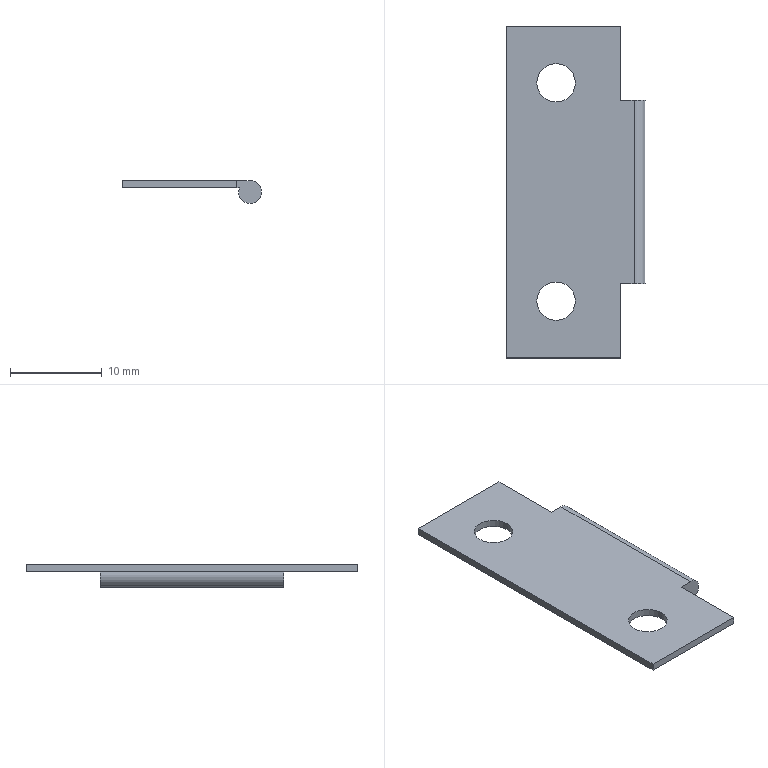Part | STEP file | 1.5 inch micro hinge plate-right | 1 solid | 15 faces | box 15.15 x 36.2 x 2.5 mm | volume 446.218 mm3 | plane 9 | cylinder 6 | commonest cylinder face diameters 4.2 x4 2.5 x2
STEP:
#1=CARTESIAN_POINT('',(0.,0.,0.));
#2=DIRECTION('',(0.,0.,1.));
#3=DIRECTION('',(1.,0.,0.));
#4=AXIS2_PLACEMENT_3D('',#1,#2,#3);
#5=CARTESIAN_POINT('',(-3.65,11.9,0.4));
#6=VERTEX_POINT('',#5);
#7=CARTESIAN_POINT('',(-3.65,11.9,-0.4));
#8=VERTEX_POINT('',#7);
#9=CARTESIAN_POINT('',(-3.65,11.9,-0.4));
#10=DIRECTION('',(0.,0.,-1.));
#11=VECTOR('',#10,1.);
#12=LINE('',#9,#11);
#13=CARTESIAN_POINT('',(-1.55,11.9,-0.4));
#14=DIRECTION('',(0.,0.,-1.));
#15=DIRECTION('',(-1.,0.,0.));
#16=AXIS2_PLACEMENT_3D('',#13,#14,#15);
#17=CYLINDRICAL_SURFACE('',#16,2.1);
#18=CARTESIAN_POINT('',(6.283,0.));
#19=DIRECTION('',(0.,1.));
#20=VECTOR('',#19,1.);
#21=LINE('',#18,#20);
#22=(GEOMETRIC_REPRESENTATION_CONTEXT(2)PARAMETRIC_REPRESENTATION_CONTEXT()REPRESENTATION_CONTEXT('',''));
#23=DEFINITIONAL_REPRESENTATION('',(#21),#22);
#24=PCURVE('',#17,#23);
#25=CARTESIAN_POINT('',(-1.55,11.9,-0.4));
#26=DIRECTION('',(0.,0.,-1.));
#27=DIRECTION('',(-1.,0.,0.));
#28=AXIS2_PLACEMENT_3D('',#25,#26,#27);
#29=CYLINDRICAL_SURFACE('',#28,2.1);
#30=CARTESIAN_POINT('',(0.,0.));
#31=DIRECTION('',(0.,1.));
#32=VECTOR('',#31,1.);
#33=LINE('',#30,#32);
#34=(GEOMETRIC_REPRESENTATION_CONTEXT(2)PARAMETRIC_REPRESENTATION_CONTEXT()REPRESENTATION_CONTEXT('',''));
#35=DEFINITIONAL_REPRESENTATION('',(#33),#34);
#36=PCURVE('',#29,#35);
#37=SURFACE_CURVE('',#12,(#24,#36),.PCURVE_S1.);
#38=EDGE_CURVE('',#6,#8,#37,.T.);
#39=ORIENTED_EDGE('',*,*,#38,.T.);
#40=CARTESIAN_POINT('',(0.55,11.9,-0.4));
#41=VERTEX_POINT('',#40);
#42=CARTESIAN_POINT('',(-1.55,11.9,-0.4));
#43=DIRECTION('',(0.,0.,-1.));
#44=DIRECTION('',(-1.,0.,0.));
#45=AXIS2_PLACEMENT_3D('',#42,#43,#44);
#46=CIRCLE('',#45,2.1);
#47=CARTESIAN_POINT('',(0.,0.));
#48=DIRECTION('',(1.,0.));
#49=VECTOR('',#48,1.);
#50=LINE('',#47,#49);
#51=(GEOMETRIC_REPRESENTATION_CONTEXT(2)PARAMETRIC_REPRESENTATION_CONTEXT()REPRESENTATION_CONTEXT('',''));
#52=DEFINITIONAL_REPRESENTATION('',(#50),#51);
#53=PCURVE('',#17,#52);
#54=CARTESIAN_POINT('',(0.,0.,-0.4));
#55=DIRECTION('',(0.,0.,-1.));
#56=DIRECTION('',(-1.,0.,0.));
#57=AXIS2_PLACEMENT_3D('',#54,#55,#56);
#58=PLANE('',#57);
#59=CARTESIAN_POINT('',(1.55,11.9));
#60=DIRECTION('',(1.,0.));
#61=AXIS2_PLACEMENT_2D('',#59,#60);
#62=CIRCLE('',#61,2.1);
#63=(GEOMETRIC_REPRESENTATION_CONTEXT(2)PARAMETRIC_REPRESENTATION_CONTEXT()REPRESENTATION_CONTEXT('',''));
#64=DEFINITIONAL_REPRESENTATION('',(#62),#63);
#65=PCURVE('',#58,#64);
#66=SURFACE_CURVE('',#46,(#53,#65),.PCURVE_S1.);
#67=EDGE_CURVE('',#41,#8,#66,.T.);
#68=ORIENTED_EDGE('',*,*,#67,.F.);
#69=CARTESIAN_POINT('',(0.55,11.9,0.4));
#70=VERTEX_POINT('',#69);
#71=CARTESIAN_POINT('',(0.55,11.9,-0.4));
#72=DIRECTION('',(0.,0.,-1.));
#73=VECTOR('',#72,1.);
#74=LINE('',#71,#73);
#75=CARTESIAN_POINT('',(3.142,0.));
#76=DIRECTION('',(0.,1.));
#77=VECTOR('',#76,1.);
#78=LINE('',#75,#77);
#79=(GEOMETRIC_REPRESENTATION_CONTEXT(2)PARAMETRIC_REPRESENTATION_CONTEXT()REPRESENTATION_CONTEXT('',''));
#80=DEFINITIONAL_REPRESENTATION('',(#78),#79);
#81=PCURVE('',#17,#80);
#82=CARTESIAN_POINT('',(3.142,0.));
#83=DIRECTION('',(0.,1.));
#84=VECTOR('',#83,1.);
#85=LINE('',#82,#84);
#86=(GEOMETRIC_REPRESENTATION_CONTEXT(2)PARAMETRIC_REPRESENTATION_CONTEXT()REPRESENTATION_CONTEXT('',''));
#87=DEFINITIONAL_REPRESENTATION('',(#85),#86);
#88=PCURVE('',#29,#87);
#89=SURFACE_CURVE('',#74,(#81,#88),.PCURVE_S1.);
#90=EDGE_CURVE('',#70,#41,#89,.T.);
#91=ORIENTED_EDGE('',*,*,#90,.F.);
#92=CARTESIAN_POINT('',(-1.55,11.9,0.4));
#93=DIRECTION('',(0.,0.,-1.));
#94=DIRECTION('',(-1.,0.,0.));
#95=AXIS2_PLACEMENT_3D('',#92,#93,#94);
#96=CIRCLE('',#95,2.1);
#97=CARTESIAN_POINT('',(0.,-0.8));
#98=DIRECTION('',(1.,0.));
#99=VECTOR('',#98,1.);
#100=LINE('',#97,#99);
#101=(GEOMETRIC_REPRESENTATION_CONTEXT(2)PARAMETRIC_REPRESENTATION_CONTEXT()REPRESENTATION_CONTEXT('',''));
#102=DEFINITIONAL_REPRESENTATION('',(#100),#101);
#103=PCURVE('',#17,#102);
#104=CARTESIAN_POINT('',(0.,0.,0.4));
#105=DIRECTION('',(0.,0.,-1.));
#106=DIRECTION('',(-1.,0.,0.));
#107=AXIS2_PLACEMENT_3D('',#104,#105,#106);
#108=PLANE('',#107);
#109=CARTESIAN_POINT('',(1.55,11.9));
#110=DIRECTION('',(1.,0.));
#111=AXIS2_PLACEMENT_2D('',#109,#110);
#112=CIRCLE('',#111,2.1);
#113=(GEOMETRIC_REPRESENTATION_CONTEXT(2)PARAMETRIC_REPRESENTATION_CONTEXT()REPRESENTATION_CONTEXT('',''));
#114=DEFINITIONAL_REPRESENTATION('',(#112),#113);
#115=PCURVE('',#108,#114);
#116=SURFACE_CURVE('',#96,(#103,#115),.PCURVE_S1.);
#117=EDGE_CURVE('',#70,#6,#116,.T.);
#118=ORIENTED_EDGE('',*,*,#117,.T.);
#119=EDGE_LOOP('',(#39,#68,#91,#118));
#120=FACE_BOUND('',#119,.F.);
#121=ADVANCED_FACE('',(#120),#17,.F.);
#122=CARTESIAN_POINT('',(-3.65,-11.9,0.4));
#123=VERTEX_POINT('',#122);
#124=CARTESIAN_POINT('',(-3.65,-11.9,-0.4));
#125=VERTEX_POINT('',#124);
#126=CARTESIAN_POINT('',(-3.65,-11.9,-0.4));
#127=DIRECTION('',(0.,0.,-1.));
#128=VECTOR('',#127,1.);
#129=LINE('',#126,#128);
#130=CARTESIAN_POINT('',(-1.55,-11.9,-0.4));
#131=DIRECTION('',(0.,0.,-1.));
#132=DIRECTION('',(-1.,0.,0.));
#133=AXIS2_PLACEMENT_3D('',#130,#131,#132);
#134=CYLINDRICAL_SURFACE('',#133,2.1);
#135=CARTESIAN_POINT('',(6.283,0.));
#136=DIRECTION('',(0.,1.));
#137=VECTOR('',#136,1.);
#138=LINE('',#135,#137);
#139=(GEOMETRIC_REPRESENTATION_CONTEXT(2)PARAMETRIC_REPRESENTATION_CONTEXT()REPRESENTATION_CONTEXT('',''));
#140=DEFINITIONAL_REPRESENTATION('',(#138),#139);
#141=PCURVE('',#134,#140);
#142=CARTESIAN_POINT('',(-1.55,-11.9,-0.4));
#143=DIRECTION('',(0.,0.,-1.));
#144=DIRECTION('',(-1.,0.,0.));
#145=AXIS2_PLACEMENT_3D('',#142,#143,#144);
#146=CYLINDRICAL_SURFACE('',#145,2.1);
#147=CARTESIAN_POINT('',(0.,0.));
#148=DIRECTION('',(0.,1.));
#149=VECTOR('',#148,1.);
#150=LINE('',#147,#149);
#151=(GEOMETRIC_REPRESENTATION_CONTEXT(2)PARAMETRIC_REPRESENTATION_CONTEXT()REPRESENTATION_CONTEXT('',''));
#152=DEFINITIONAL_REPRESENTATION('',(#150),#151);
#153=PCURVE('',#146,#152);
#154=SURFACE_CURVE('',#129,(#141,#153),.PCURVE_S1.);
#155=EDGE_CURVE('',#123,#125,#154,.T.);
#156=ORIENTED_EDGE('',*,*,#155,.T.);
#157=CARTESIAN_POINT('',(0.55,-11.9,-0.4));
#158=VERTEX_POINT('',#157);
#159=CARTESIAN_POINT('',(-1.55,-11.9,-0.4));
#160=DIRECTION('',(0.,0.,-1.));
#161=DIRECTION('',(-1.,0.,0.));
#162=AXIS2_PLACEMENT_3D('',#159,#160,#161);
#163=CIRCLE('',#162,2.1);
#164=CARTESIAN_POINT('',(0.,0.));
#165=DIRECTION('',(1.,0.));
#166=VECTOR('',#165,1.);
#167=LINE('',#164,#166);
#168=(GEOMETRIC_REPRESENTATION_CONTEXT(2)PARAMETRIC_REPRESENTATION_CONTEXT()REPRESENTATION_CONTEXT('',''));
#169=DEFINITIONAL_REPRESENTATION('',(#167),#168);
#170=PCURVE('',#134,#169);
#171=CARTESIAN_POINT('',(1.55,-11.9));
#172=DIRECTION('',(1.,0.));
#173=AXIS2_PLACEMENT_2D('',#171,#172);
#174=CIRCLE('',#173,2.1);
#175=(GEOMETRIC_REPRESENTATION_CONTEXT(2)PARAMETRIC_REPRESENTATION_CONTEXT()REPRESENTATION_CONTEXT('',''));
#176=DEFINITIONAL_REPRESENTATION('',(#174),#175);
#177=PCURVE('',#58,#176);
#178=SURFACE_CURVE('',#163,(#170,#177),.PCURVE_S1.);
#179=EDGE_CURVE('',#158,#125,#178,.T.);
#180=ORIENTED_EDGE('',*,*,#179,.F.);
#181=CARTESIAN_POINT('',(0.55,-11.9,0.4));
#182=VERTEX_POINT('',#181);
#183=CARTESIAN_POINT('',(0.55,-11.9,-0.4));
#184=DIRECTION('',(0.,0.,-1.));
#185=VECTOR('',#184,1.);
#186=LINE('',#183,#185);
#187=CARTESIAN_POINT('',(3.142,0.));
#188=DIRECTION('',(0.,1.));
#189=VECTOR('',#188,1.);
#190=LINE('',#187,#189);
#191=(GEOMETRIC_REPRESENTATION_CONTEXT(2)PARAMETRIC_REPRESENTATION_CONTEXT()REPRESENTATION_CONTEXT('',''));
#192=DEFINITIONAL_REPRESENTATION('',(#190),#191);
#193=PCURVE('',#134,#192);
#194=CARTESIAN_POINT('',(3.142,0.));
#195=DIRECTION('',(0.,1.));
#196=VECTOR('',#195,1.);
#197=LINE('',#194,#196);
#198=(GEOMETRIC_REPRESENTATION_CONTEXT(2)PARAMETRIC_REPRESENTATION_CONTEXT()REPRESENTATION_CONTEXT('',''));
#199=DEFINITIONAL_REPRESENTATION('',(#197),#198);
#200=PCURVE('',#146,#199);
#201=SURFACE_CURVE('',#186,(#193,#200),.PCURVE_S1.);
#202=EDGE_CURVE('',#182,#158,#201,.T.);
#203=ORIENTED_EDGE('',*,*,#202,.F.);
#204=CARTESIAN_POINT('',(-1.55,-11.9,0.4));
#205=DIRECTION('',(0.,0.,-1.));
#206=DIRECTION('',(-1.,0.,0.));
#207=AXIS2_PLACEMENT_3D('',#204,#205,#206);
#208=CIRCLE('',#207,2.1);
#209=CARTESIAN_POINT('',(0.,-0.8));
#210=DIRECTION('',(1.,0.));
#211=VECTOR('',#210,1.);
#212=LINE('',#209,#211);
#213=(GEOMETRIC_REPRESENTATION_CONTEXT(2)PARAMETRIC_REPRESENTATION_CONTEXT()REPRESENTATION_CONTEXT('',''));
#214=DEFINITIONAL_REPRESENTATION('',(#212),#213);
#215=PCURVE('',#134,#214);
#216=CARTESIAN_POINT('',(1.55,-11.9));
#217=DIRECTION('',(1.,0.));
#218=AXIS2_PLACEMENT_2D('',#216,#217);
#219=CIRCLE('',#218,2.1);
#220=(GEOMETRIC_REPRESENTATION_CONTEXT(2)PARAMETRIC_REPRESENTATION_CONTEXT()REPRESENTATION_CONTEXT('',''));
#221=DEFINITIONAL_REPRESENTATION('',(#219),#220);
#222=PCURVE('',#108,#221);
#223=SURFACE_CURVE('',#208,(#215,#222),.PCURVE_S1.);
#224=EDGE_CURVE('',#182,#123,#223,.T.);
#225=ORIENTED_EDGE('',*,*,#224,.T.);
#226=EDGE_LOOP('',(#156,#180,#203,#225));
#227=FACE_BOUND('',#226,.F.);
#228=ADVANCED_FACE('',(#227),#134,.F.);
#229=CARTESIAN_POINT('',(6.95,10.,-2.1));
#230=VERTEX_POINT('',#229);
#231=CARTESIAN_POINT('',(5.784,10.,-0.4));
#232=VERTEX_POINT('',#231);
#233=CARTESIAN_POINT('',(6.95,10.,-0.85));
#234=DIRECTION('',(0.,1.,0.));
#235=DIRECTION('',(0.,0.,1.));
#236=AXIS2_PLACEMENT_3D('',#233,#234,#235);
#237=CIRCLE('',#236,1.25);
#238=CARTESIAN_POINT('',(6.95,18.1,-0.85));
#239=DIRECTION('',(0.,-1.,0.));
#240=DIRECTION('',(0.,0.,-1.));
#241=AXIS2_PLACEMENT_3D('',#238,#239,#240);
#242=CYLINDRICAL_SURFACE('',#241,1.25);
#243=CARTESIAN_POINT('',(9.425,8.1));
#244=DIRECTION('',(-1.,0.));
#245=VECTOR('',#244,1.);
#246=LINE('',#243,#245);
#247=(GEOMETRIC_REPRESENTATION_CONTEXT(2)PARAMETRIC_REPRESENTATION_CONTEXT()REPRESENTATION_CONTEXT('',''));
#248=DEFINITIONAL_REPRESENTATION('',(#246),#247);
#249=PCURVE('',#242,#248);
#250=CARTESIAN_POINT('',(5.5,10.,0.4));
#251=DIRECTION('',(0.,1.,0.));
#252=DIRECTION('',(0.,0.,1.));
#253=AXIS2_PLACEMENT_3D('',#250,#251,#252);
#254=PLANE('',#253);
#255=CARTESIAN_POINT('',(-1.25,1.45));
#256=DIRECTION('',(1.,0.));
#257=AXIS2_PLACEMENT_2D('',#255,#256);
#258=CIRCLE('',#257,1.25);
#259=(GEOMETRIC_REPRESENTATION_CONTEXT(2)PARAMETRIC_REPRESENTATION_CONTEXT()REPRESENTATION_CONTEXT('',''));
#260=DEFINITIONAL_REPRESENTATION('',(#258),#259);
#261=PCURVE('',#254,#260);
#262=SURFACE_CURVE('',#237,(#249,#261),.PCURVE_S1.);
#263=EDGE_CURVE('',#230,#232,#262,.T.);
#264=ORIENTED_EDGE('',*,*,#263,.F.);
#265=CARTESIAN_POINT('',(6.95,-10.,-2.1));
#266=VERTEX_POINT('',#265);
#267=CARTESIAN_POINT('',(6.95,18.1,-2.1));
#268=DIRECTION('',(0.,-1.,0.));
#269=VECTOR('',#268,1.);
#270=LINE('',#267,#269);
#271=CARTESIAN_POINT('',(6.283,0.));
#272=DIRECTION('',(0.,1.));
#273=VECTOR('',#272,1.);
#274=LINE('',#271,#273);
#275=(GEOMETRIC_REPRESENTATION_CONTEXT(2)PARAMETRIC_REPRESENTATION_CONTEXT()REPRESENTATION_CONTEXT('',''));
#276=DEFINITIONAL_REPRESENTATION('',(#274),#275);
#277=PCURVE('',#242,#276);
#278=CARTESIAN_POINT('',(6.95,18.1,-0.85));
#279=DIRECTION('',(0.,-1.,0.));
#280=DIRECTION('',(0.,0.,-1.));
#281=AXIS2_PLACEMENT_3D('',#278,#279,#280);
#282=CYLINDRICAL_SURFACE('',#281,1.25);
#283=CARTESIAN_POINT('',(0.,0.));
#284=DIRECTION('',(0.,1.));
#285=VECTOR('',#284,1.);
#286=LINE('',#283,#285);
#287=(GEOMETRIC_REPRESENTATION_CONTEXT(2)PARAMETRIC_REPRESENTATION_CONTEXT()REPRESENTATION_CONTEXT('',''));
#288=DEFINITIONAL_REPRESENTATION('',(#286),#287);
#289=PCURVE('',#282,#288);
#290=SURFACE_CURVE('',#270,(#277,#289),.PCURVE_S1.);
#291=EDGE_CURVE('',#230,#266,#290,.T.);
#292=ORIENTED_EDGE('',*,*,#291,.T.);
#293=CARTESIAN_POINT('',(5.784,-10.,-0.4));
#294=VERTEX_POINT('',#293);
#295=CARTESIAN_POINT('',(6.95,-10.,-0.85));
#296=DIRECTION('',(0.,-1.,0.));
#297=DIRECTION('',(0.,0.,-1.));
#298=AXIS2_PLACEMENT_3D('',#295,#296,#297);
#299=CIRCLE('',#298,1.25);
#300=CARTESIAN_POINT('',(0.,28.1));
#301=DIRECTION('',(1.,0.));
#302=VECTOR('',#301,1.);
#303=LINE('',#300,#302);
#304=(GEOMETRIC_REPRESENTATION_CONTEXT(2)PARAMETRIC_REPRESENTATION_CONTEXT()REPRESENTATION_CONTEXT('',''));
#305=DEFINITIONAL_REPRESENTATION('',(#303),#304);
#306=PCURVE('',#242,#305);
#307=CARTESIAN_POINT('',(5.5,-10.,0.4));
#308=DIRECTION('',(0.,-1.,0.));
#309=DIRECTION('',(0.,0.,-1.));
#310=AXIS2_PLACEMENT_3D('',#307,#308,#309);
#311=PLANE('',#310);
#312=CARTESIAN_POINT('',(1.25,1.45));
#313=DIRECTION('',(1.,0.));
#314=AXIS2_PLACEMENT_2D('',#312,#313);
#315=CIRCLE('',#314,1.25);
#316=(GEOMETRIC_REPRESENTATION_CONTEXT(2)PARAMETRIC_REPRESENTATION_CONTEXT()REPRESENTATION_CONTEXT('',''));
#317=DEFINITIONAL_REPRESENTATION('',(#315),#316);
#318=PCURVE('',#311,#317);
#319=SURFACE_CURVE('',#299,(#306,#318),.PCURVE_S1.);
#320=EDGE_CURVE('',#294,#266,#319,.T.);
#321=ORIENTED_EDGE('',*,*,#320,.F.);
#322=CARTESIAN_POINT('',(5.784,18.1,-0.4));
#323=DIRECTION('',(0.,-1.,0.));
#324=VECTOR('',#323,1.);
#325=LINE('',#322,#324);
#326=CARTESIAN_POINT('',(4.344,0.));
#327=DIRECTION('',(0.,1.));
#328=VECTOR('',#327,1.);
#329=LINE('',#326,#328);
#330=(GEOMETRIC_REPRESENTATION_CONTEXT(2)PARAMETRIC_REPRESENTATION_CONTEXT()REPRESENTATION_CONTEXT('',''));
#331=DEFINITIONAL_REPRESENTATION('',(#329),#330);
#332=PCURVE('',#242,#331);
#333=CARTESIAN_POINT('',(-5.784,18.1));
#334=DIRECTION('',(0.,-1.));
#335=VECTOR('',#334,1.);
#336=LINE('',#333,#335);
#337=(GEOMETRIC_REPRESENTATION_CONTEXT(2)PARAMETRIC_REPRESENTATION_CONTEXT()REPRESENTATION_CONTEXT('',''));
#338=DEFINITIONAL_REPRESENTATION('',(#336),#337);
#339=PCURVE('',#58,#338);
#340=SURFACE_CURVE('',#325,(#332,#339),.PCURVE_S1.);
#341=EDGE_CURVE('',#232,#294,#340,.T.);
#342=ORIENTED_EDGE('',*,*,#341,.F.);
#343=EDGE_LOOP('',(#264,#292,#321,#342));
#344=FACE_BOUND('',#343,.T.);
#345=ADVANCED_FACE('',(#344),#242,.T.);
#346=CARTESIAN_POINT('',(-1.55,11.9,-0.4));
#347=DIRECTION('',(0.,0.,-1.));
#348=DIRECTION('',(-1.,0.,0.));
#349=AXIS2_PLACEMENT_3D('',#346,#347,#348);
#350=CIRCLE('',#349,2.1);
#351=CARTESIAN_POINT('',(1.55,11.9));
#352=DIRECTION('',(1.,0.));
#353=AXIS2_PLACEMENT_2D('',#351,#352);
#354=CIRCLE('',#353,2.1);
#355=(GEOMETRIC_REPRESENTATION_CONTEXT(2)PARAMETRIC_REPRESENTATION_CONTEXT()REPRESENTATION_CONTEXT('',''));
#356=DEFINITIONAL_REPRESENTATION('',(#354),#355);
#357=PCURVE('',#58,#356);
#358=CARTESIAN_POINT('',(0.,0.));
#359=DIRECTION('',(1.,0.));
#360=VECTOR('',#359,1.);
#361=LINE('',#358,#360);
#362=(GEOMETRIC_REPRESENTATION_CONTEXT(2)PARAMETRIC_REPRESENTATION_CONTEXT()REPRESENTATION_CONTEXT('',''));
#363=DEFINITIONAL_REPRESENTATION('',(#361),#362);
#364=PCURVE('',#29,#363);
#365=SURFACE_CURVE('',#350,(#357,#364),.PCURVE_S1.);
#366=EDGE_CURVE('',#8,#41,#365,.T.);
#367=ORIENTED_EDGE('',*,*,#366,.F.);
#368=ORIENTED_EDGE('',*,*,#67,.F.);
#369=EDGE_LOOP('',(#367,#368));
#370=FACE_BOUND('',#369,.T.);
#371=CARTESIAN_POINT('',(-1.55,-11.9,-0.4));
#372=DIRECTION('',(0.,0.,-1.));
#373=DIRECTION('',(-1.,0.,0.));
#374=AXIS2_PLACEMENT_3D('',#371,#372,#373);
#375=CIRCLE('',#374,2.1);
#376=CARTESIAN_POINT('',(1.55,-11.9));
#377=DIRECTION('',(1.,0.));
#378=AXIS2_PLACEMENT_2D('',#376,#377);
#379=CIRCLE('',#378,2.1);
#380=(GEOMETRIC_REPRESENTATION_CONTEXT(2)PARAMETRIC_REPRESENTATION_CONTEXT()REPRESENTATION_CONTEXT('',''));
#381=DEFINITIONAL_REPRESENTATION('',(#379),#380);
#382=PCURVE('',#58,#381);
#383=CARTESIAN_POINT('',(0.,0.));
#384=DIRECTION('',(1.,0.));
#385=VECTOR('',#384,1.);
#386=LINE('',#383,#385);
#387=(GEOMETRIC_REPRESENTATION_CONTEXT(2)PARAMETRIC_REPRESENTATION_CONTEXT()REPRESENTATION_CONTEXT('',''));
#388=DEFINITIONAL_REPRESENTATION('',(#386),#387);
#389=PCURVE('',#146,#388);
#390=SURFACE_CURVE('',#375,(#382,#389),.PCURVE_S1.);
#391=EDGE_CURVE('',#125,#158,#390,.T.);
#392=ORIENTED_EDGE('',*,*,#391,.F.);
#393=ORIENTED_EDGE('',*,*,#179,.F.);
#394=EDGE_LOOP('',(#392,#393));
#395=FACE_BOUND('',#394,.T.);
#396=CARTESIAN_POINT('',(5.5,-10.,-0.4));
#397=VERTEX_POINT('',#396);
#398=CARTESIAN_POINT('',(0.,-10.,-0.4));
#399=DIRECTION('',(-1.,0.,0.));
#400=VECTOR('',#399,1.);
#401=LINE('',#398,#400);
#402=CARTESIAN_POINT('',(0.,-10.));
#403=DIRECTION('',(1.,0.));
#404=VECTOR('',#403,1.);
#405=LINE('',#402,#404);
#406=(GEOMETRIC_REPRESENTATION_CONTEXT(2)PARAMETRIC_REPRESENTATION_CONTEXT()REPRESENTATION_CONTEXT('',''));
#407=DEFINITIONAL_REPRESENTATION('',(#405),#406);
#408=PCURVE('',#58,#407);
#409=CARTESIAN_POINT('',(0.8,-5.5));
#410=DIRECTION('',(0.,-1.));
#411=VECTOR('',#410,1.);
#412=LINE('',#409,#411);
#413=(GEOMETRIC_REPRESENTATION_CONTEXT(2)PARAMETRIC_REPRESENTATION_CONTEXT()REPRESENTATION_CONTEXT('',''));
#414=DEFINITIONAL_REPRESENTATION('',(#412),#413);
#415=PCURVE('',#311,#414);
#416=SURFACE_CURVE('',#401,(#408,#415),.PCURVE_S1.);
#417=EDGE_CURVE('',#294,#397,#416,.T.);
#418=ORIENTED_EDGE('',*,*,#417,.T.);
#419=CARTESIAN_POINT('',(5.5,-18.1,-0.4));
#420=VERTEX_POINT('',#419);
#421=CARTESIAN_POINT('',(5.5,0.,-0.4));
#422=DIRECTION('',(0.,-1.,0.));
#423=VECTOR('',#422,1.);
#424=LINE('',#421,#423);
#425=CARTESIAN_POINT('',(-5.5,0.));
#426=DIRECTION('',(0.,-1.));
#427=VECTOR('',#426,1.);
#428=LINE('',#425,#427);
#429=(GEOMETRIC_REPRESENTATION_CONTEXT(2)PARAMETRIC_REPRESENTATION_CONTEXT()REPRESENTATION_CONTEXT('',''));
#430=DEFINITIONAL_REPRESENTATION('',(#428),#429);
#431=PCURVE('',#58,#430);
#432=CARTESIAN_POINT('',(5.5,0.,-3.651));
#433=DIRECTION('',(1.,0.,0.));
#434=DIRECTION('',(0.,0.,-1.));
#435=AXIS2_PLACEMENT_3D('',#432,#433,#434);
#436=PLANE('',#435);
#437=CARTESIAN_POINT('',(-3.251,0.));
#438=DIRECTION('',(0.,-1.));
#439=VECTOR('',#438,1.);
#440=LINE('',#437,#439);
#441=(GEOMETRIC_REPRESENTATION_CONTEXT(2)PARAMETRIC_REPRESENTATION_CONTEXT()REPRESENTATION_CONTEXT('',''));
#442=DEFINITIONAL_REPRESENTATION('',(#440),#441);
#443=PCURVE('',#436,#442);
#444=SURFACE_CURVE('',#424,(#431,#443),.PCURVE_S1.);
#445=EDGE_CURVE('',#397,#420,#444,.T.);
#446=ORIENTED_EDGE('',*,*,#445,.T.);
#447=CARTESIAN_POINT('',(-6.95,-18.1,-0.4));
#448=VERTEX_POINT('',#447);
#449=CARTESIAN_POINT('',(-6.95,-18.1,-0.4));
#450=DIRECTION('',(1.,0.,0.));
#451=VECTOR('',#450,1.);
#452=LINE('',#449,#451);
#453=CARTESIAN_POINT('',(6.95,-18.1));
#454=DIRECTION('',(-1.,0.));
#455=VECTOR('',#454,1.);
#456=LINE('',#453,#455);
#457=(GEOMETRIC_REPRESENTATION_CONTEXT(2)PARAMETRIC_REPRESENTATION_CONTEXT()REPRESENTATION_CONTEXT('',''));
#458=DEFINITIONAL_REPRESENTATION('',(#456),#457);
#459=PCURVE('',#58,#458);
#460=CARTESIAN_POINT('',(-6.95,-18.1,0.4));
#461=DIRECTION('',(0.,1.,0.));
#462=DIRECTION('',(0.,0.,1.));
#463=AXIS2_PLACEMENT_3D('',#460,#461,#462);
#464=PLANE('',#463);
#465=CARTESIAN_POINT('',(-0.8,0.));
#466=DIRECTION('',(0.,1.));
#467=VECTOR('',#466,1.);
#468=LINE('',#465,#467);
#469=(GEOMETRIC_REPRESENTATION_CONTEXT(2)PARAMETRIC_REPRESENTATION_CONTEXT()REPRESENTATION_CONTEXT('',''));
#470=DEFINITIONAL_REPRESENTATION('',(#468),#469);
#471=PCURVE('',#464,#470);
#472=SURFACE_CURVE('',#452,(#459,#471),.PCURVE_S1.);
#473=EDGE_CURVE('',#448,#420,#472,.T.);
#474=ORIENTED_EDGE('',*,*,#473,.F.);
#475=CARTESIAN_POINT('',(-6.95,18.1,-0.4));
#476=VERTEX_POINT('',#475);
#477=CARTESIAN_POINT('',(-6.95,-18.1,-0.4));
#478=DIRECTION('',(0.,-1.,0.));
#479=VECTOR('',#478,1.);
#480=LINE('',#477,#479);
#481=CARTESIAN_POINT('',(6.95,-18.1));
#482=DIRECTION('',(0.,-1.));
#483=VECTOR('',#482,1.);
#484=LINE('',#481,#483);
#485=(GEOMETRIC_REPRESENTATION_CONTEXT(2)PARAMETRIC_REPRESENTATION_CONTEXT()REPRESENTATION_CONTEXT('',''));
#486=DEFINITIONAL_REPRESENTATION('',(#484),#485);
#487=PCURVE('',#58,#486);
#488=CARTESIAN_POINT('',(-6.95,-18.1,0.4));
#489=DIRECTION('',(1.,0.,0.));
#490=DIRECTION('',(0.,0.,-1.));
#491=AXIS2_PLACEMENT_3D('',#488,#489,#490);
#492=PLANE('',#491);
#493=CARTESIAN_POINT('',(0.8,0.));
#494=DIRECTION('',(0.,-1.));
#495=VECTOR('',#494,1.);
#496=LINE('',#493,#495);
#497=(GEOMETRIC_REPRESENTATION_CONTEXT(2)PARAMETRIC_REPRESENTATION_CONTEXT()REPRESENTATION_CONTEXT('',''));
#498=DEFINITIONAL_REPRESENTATION('',(#496),#497);
#499=PCURVE('',#492,#498);
#500=SURFACE_CURVE('',#480,(#487,#499),.PCURVE_S1.);
#501=EDGE_CURVE('',#476,#448,#500,.T.);
#502=ORIENTED_EDGE('',*,*,#501,.F.);
#503=CARTESIAN_POINT('',(5.5,18.1,-0.4));
#504=VERTEX_POINT('',#503);
#505=CARTESIAN_POINT('',(-6.95,18.1,-0.4));
#506=DIRECTION('',(-1.,0.,0.));
#507=VECTOR('',#506,1.);
#508=LINE('',#505,#507);
#509=CARTESIAN_POINT('',(6.95,18.1));
#510=DIRECTION('',(1.,0.));
#511=VECTOR('',#510,1.);
#512=LINE('',#509,#511);
#513=(GEOMETRIC_REPRESENTATION_CONTEXT(2)PARAMETRIC_REPRESENTATION_CONTEXT()REPRESENTATION_CONTEXT('',''));
#514=DEFINITIONAL_REPRESENTATION('',(#512),#513);
#515=PCURVE('',#58,#514);
#516=CARTESIAN_POINT('',(-6.95,18.1,0.4));
#517=DIRECTION('',(0.,-1.,0.));
#518=DIRECTION('',(0.,0.,-1.));
#519=AXIS2_PLACEMENT_3D('',#516,#517,#518);
#520=PLANE('',#519);
#521=CARTESIAN_POINT('',(0.8,0.));
#522=DIRECTION('',(0.,-1.));
#523=VECTOR('',#522,1.);
#524=LINE('',#521,#523);
#525=(GEOMETRIC_REPRESENTATION_CONTEXT(2)PARAMETRIC_REPRESENTATION_CONTEXT()REPRESENTATION_CONTEXT('',''));
#526=DEFINITIONAL_REPRESENTATION('',(#524),#525);
#527=PCURVE('',#520,#526);
#528=SURFACE_CURVE('',#508,(#515,#527),.PCURVE_S1.);
#529=EDGE_CURVE('',#504,#476,#528,.T.);
#530=ORIENTED_EDGE('',*,*,#529,.F.);
#531=CARTESIAN_POINT('',(5.5,10.,-0.4));
#532=VERTEX_POINT('',#531);
#533=CARTESIAN_POINT('',(5.5,0.,-0.4));
#534=DIRECTION('',(0.,-1.,0.));
#535=VECTOR('',#534,1.);
#536=LINE('',#533,#535);
#537=CARTESIAN_POINT('',(-5.5,0.));
#538=DIRECTION('',(0.,-1.));
#539=VECTOR('',#538,1.);
#540=LINE('',#537,#539);
#541=(GEOMETRIC_REPRESENTATION_CONTEXT(2)PARAMETRIC_REPRESENTATION_CONTEXT()REPRESENTATION_CONTEXT('',''));
#542=DEFINITIONAL_REPRESENTATION('',(#540),#541);
#543=PCURVE('',#58,#542);
#544=CARTESIAN_POINT('',(5.5,0.,-3.651));
#545=DIRECTION('',(1.,0.,0.));
#546=DIRECTION('',(0.,0.,-1.));
#547=AXIS2_PLACEMENT_3D('',#544,#545,#546);
#548=PLANE('',#547);
#549=CARTESIAN_POINT('',(-3.251,0.));
#550=DIRECTION('',(0.,-1.));
#551=VECTOR('',#550,1.);
#552=LINE('',#549,#551);
#553=(GEOMETRIC_REPRESENTATION_CONTEXT(2)PARAMETRIC_REPRESENTATION_CONTEXT()REPRESENTATION_CONTEXT('',''));
#554=DEFINITIONAL_REPRESENTATION('',(#552),#553);
#555=PCURVE('',#548,#554);
#556=SURFACE_CURVE('',#536,(#543,#555),.PCURVE_S1.);
#557=EDGE_CURVE('',#504,#532,#556,.T.);
#558=ORIENTED_EDGE('',*,*,#557,.T.);
#559=CARTESIAN_POINT('',(0.,10.,-0.4));
#560=DIRECTION('',(1.,0.,0.));
#561=VECTOR('',#560,1.);
#562=LINE('',#559,#561);
#563=CARTESIAN_POINT('',(0.,10.));
#564=DIRECTION('',(-1.,0.));
#565=VECTOR('',#564,1.);
#566=LINE('',#563,#565);
#567=(GEOMETRIC_REPRESENTATION_CONTEXT(2)PARAMETRIC_REPRESENTATION_CONTEXT()REPRESENTATION_CONTEXT('',''));
#568=DEFINITIONAL_REPRESENTATION('',(#566),#567);
#569=PCURVE('',#58,#568);
#570=CARTESIAN_POINT('',(-0.8,-5.5));
#571=DIRECTION('',(0.,1.));
#572=VECTOR('',#571,1.);
#573=LINE('',#570,#572);
#574=(GEOMETRIC_REPRESENTATION_CONTEXT(2)PARAMETRIC_REPRESENTATION_CONTEXT()REPRESENTATION_CONTEXT('',''));
#575=DEFINITIONAL_REPRESENTATION('',(#573),#574);
#576=PCURVE('',#254,#575);
#577=SURFACE_CURVE('',#562,(#569,#576),.PCURVE_S1.);
#578=EDGE_CURVE('',#532,#232,#577,.T.);
#579=ORIENTED_EDGE('',*,*,#578,.T.);
#580=ORIENTED_EDGE('',*,*,#341,.T.);
#581=EDGE_LOOP('',(#418,#446,#474,#502,#530,#558,#579,#580));
#582=FACE_BOUND('',#581,.T.);
#583=ADVANCED_FACE('',(#370,#395,#582),#58,.T.);
#584=CARTESIAN_POINT('',(5.5,18.1,0.4));
#585=VERTEX_POINT('',#584);
#586=CARTESIAN_POINT('',(5.5,18.1,0.4));
#587=DIRECTION('',(0.,0.,1.));
#588=VECTOR('',#587,1.);
#589=LINE('',#586,#588);
#590=CARTESIAN_POINT('',(0.,12.45));
#591=DIRECTION('',(-1.,0.));
#592=VECTOR('',#591,1.);
#593=LINE('',#590,#592);
#594=(GEOMETRIC_REPRESENTATION_CONTEXT(2)PARAMETRIC_REPRESENTATION_CONTEXT()REPRESENTATION_CONTEXT('',''));
#595=DEFINITIONAL_REPRESENTATION('',(#593),#594);
#596=PCURVE('',#520,#595);
#597=CARTESIAN_POINT('',(-4.051,18.1));
#598=DIRECTION('',(-1.,0.));
#599=VECTOR('',#598,1.);
#600=LINE('',#597,#599);
#601=(GEOMETRIC_REPRESENTATION_CONTEXT(2)PARAMETRIC_REPRESENTATION_CONTEXT()REPRESENTATION_CONTEXT('',''));
#602=DEFINITIONAL_REPRESENTATION('',(#600),#601);
#603=PCURVE('',#548,#602);
#604=SURFACE_CURVE('',#589,(#596,#603),.PCURVE_S1.);
#605=EDGE_CURVE('',#504,#585,#604,.T.);
#606=ORIENTED_EDGE('',*,*,#605,.F.);
#607=ORIENTED_EDGE('',*,*,#529,.T.);
#608=CARTESIAN_POINT('',(-6.95,18.1,0.4));
#609=VERTEX_POINT('',#608);
#610=CARTESIAN_POINT('',(-6.95,18.1,0.4));
#611=DIRECTION('',(0.,0.,-1.));
#612=VECTOR('',#611,1.);
#613=LINE('',#610,#612);
#614=CARTESIAN_POINT('',(0.,0.));
#615=DIRECTION('',(1.,0.));
#616=VECTOR('',#615,1.);
#617=LINE('',#614,#616);
#618=(GEOMETRIC_REPRESENTATION_CONTEXT(2)PARAMETRIC_REPRESENTATION_CONTEXT()REPRESENTATION_CONTEXT('',''));
#619=DEFINITIONAL_REPRESENTATION('',(#617),#618);
#620=PCURVE('',#520,#619);
#621=CARTESIAN_POINT('',(0.,36.2));
#622=DIRECTION('',(1.,0.));
#623=VECTOR('',#622,1.);
#624=LINE('',#621,#623);
#625=(GEOMETRIC_REPRESENTATION_CONTEXT(2)PARAMETRIC_REPRESENTATION_CONTEXT()REPRESENTATION_CONTEXT('',''));
#626=DEFINITIONAL_REPRESENTATION('',(#624),#625);
#627=PCURVE('',#492,#626);
#628=SURFACE_CURVE('',#613,(#620,#627),.PCURVE_S1.);
#629=EDGE_CURVE('',#609,#476,#628,.T.);
#630=ORIENTED_EDGE('',*,*,#629,.F.);
#631=CARTESIAN_POINT('',(-6.95,18.1,0.4));
#632=DIRECTION('',(-1.,0.,0.));
#633=VECTOR('',#632,1.);
#634=LINE('',#631,#633);
#635=CARTESIAN_POINT('',(0.,0.));
#636=DIRECTION('',(0.,-1.));
#637=VECTOR('',#636,1.);
#638=LINE('',#635,#637);
#639=(GEOMETRIC_REPRESENTATION_CONTEXT(2)PARAMETRIC_REPRESENTATION_CONTEXT()REPRESENTATION_CONTEXT('',''));
#640=DEFINITIONAL_REPRESENTATION('',(#638),#639);
#641=PCURVE('',#520,#640);
#642=CARTESIAN_POINT('',(6.95,18.1));
#643=DIRECTION('',(1.,0.));
#644=VECTOR('',#643,1.);
#645=LINE('',#642,#644);
#646=(GEOMETRIC_REPRESENTATION_CONTEXT(2)PARAMETRIC_REPRESENTATION_CONTEXT()REPRESENTATION_CONTEXT('',''));
#647=DEFINITIONAL_REPRESENTATION('',(#645),#646);
#648=PCURVE('',#108,#647);
#649=SURFACE_CURVE('',#634,(#641,#648),.PCURVE_S1.);
#650=EDGE_CURVE('',#585,#609,#649,.T.);
#651=ORIENTED_EDGE('',*,*,#650,.F.);
#652=EDGE_LOOP('',(#606,#607,#630,#651));
#653=FACE_BOUND('',#652,.T.);
#654=ADVANCED_FACE('',(#653),#520,.F.);
#655=CARTESIAN_POINT('',(5.5,-18.1,0.4));
#656=VERTEX_POINT('',#655);
#657=CARTESIAN_POINT('',(5.5,-18.1,0.4));
#658=DIRECTION('',(0.,0.,-1.));
#659=VECTOR('',#658,1.);
#660=LINE('',#657,#659);
#661=CARTESIAN_POINT('',(0.,12.45));
#662=DIRECTION('',(-1.,0.));
#663=VECTOR('',#662,1.);
#664=LINE('',#661,#663);
#665=(GEOMETRIC_REPRESENTATION_CONTEXT(2)PARAMETRIC_REPRESENTATION_CONTEXT()REPRESENTATION_CONTEXT('',''));
#666=DEFINITIONAL_REPRESENTATION('',(#664),#665);
#667=PCURVE('',#464,#666);
#668=CARTESIAN_POINT('',(-4.051,-18.1));
#669=DIRECTION('',(1.,0.));
#670=VECTOR('',#669,1.);
#671=LINE('',#668,#670);
#672=(GEOMETRIC_REPRESENTATION_CONTEXT(2)PARAMETRIC_REPRESENTATION_CONTEXT()REPRESENTATION_CONTEXT('',''));
#673=DEFINITIONAL_REPRESENTATION('',(#671),#672);
#674=PCURVE('',#436,#673);
#675=SURFACE_CURVE('',#660,(#667,#674),.PCURVE_S1.);
#676=EDGE_CURVE('',#656,#420,#675,.T.);
#677=ORIENTED_EDGE('',*,*,#676,.F.);
#678=CARTESIAN_POINT('',(-6.95,-18.1,0.4));
#679=VERTEX_POINT('',#678);
#680=CARTESIAN_POINT('',(-6.95,-18.1,0.4));
#681=DIRECTION('',(1.,0.,0.));
#682=VECTOR('',#681,1.);
#683=LINE('',#680,#682);
#684=CARTESIAN_POINT('',(0.,0.));
#685=DIRECTION('',(0.,1.));
#686=VECTOR('',#685,1.);
#687=LINE('',#684,#686);
#688=(GEOMETRIC_REPRESENTATION_CONTEXT(2)PARAMETRIC_REPRESENTATION_CONTEXT()REPRESENTATION_CONTEXT('',''));
#689=DEFINITIONAL_REPRESENTATION('',(#687),#688);
#690=PCURVE('',#464,#689);
#691=CARTESIAN_POINT('',(6.95,-18.1));
#692=DIRECTION('',(-1.,0.));
#693=VECTOR('',#692,1.);
#694=LINE('',#691,#693);
#695=(GEOMETRIC_REPRESENTATION_CONTEXT(2)PARAMETRIC_REPRESENTATION_CONTEXT()REPRESENTATION_CONTEXT('',''));
#696=DEFINITIONAL_REPRESENTATION('',(#694),#695);
#697=PCURVE('',#108,#696);
#698=SURFACE_CURVE('',#683,(#690,#697),.PCURVE_S1.);
#699=EDGE_CURVE('',#679,#656,#698,.T.);
#700=ORIENTED_EDGE('',*,*,#699,.F.);
#701=CARTESIAN_POINT('',(-6.95,-18.1,0.4));
#702=DIRECTION('',(0.,0.,-1.));
#703=VECTOR('',#702,1.);
#704=LINE('',#701,#703);
#705=CARTESIAN_POINT('',(0.,0.));
#706=DIRECTION('',(-1.,0.));
#707=VECTOR('',#706,1.);
#708=LINE('',#705,#707);
#709=(GEOMETRIC_REPRESENTATION_CONTEXT(2)PARAMETRIC_REPRESENTATION_CONTEXT()REPRESENTATION_CONTEXT('',''));
#710=DEFINITIONAL_REPRESENTATION('',(#708),#709);
#711=PCURVE('',#464,#710);
#712=CARTESIAN_POINT('',(0.,0.));
#713=DIRECTION('',(1.,0.));
#714=VECTOR('',#713,1.);
#715=LINE('',#712,#714);
#716=(GEOMETRIC_REPRESENTATION_CONTEXT(2)PARAMETRIC_REPRESENTATION_CONTEXT()REPRESENTATION_CONTEXT('',''));
#717=DEFINITIONAL_REPRESENTATION('',(#715),#716);
#718=PCURVE('',#492,#717);
#719=SURFACE_CURVE('',#704,(#711,#718),.PCURVE_S1.);
#720=EDGE_CURVE('',#679,#448,#719,.T.);
#721=ORIENTED_EDGE('',*,*,#720,.T.);
#722=ORIENTED_EDGE('',*,*,#473,.T.);
#723=EDGE_LOOP('',(#677,#700,#721,#722));
#724=FACE_BOUND('',#723,.T.);
#725=ADVANCED_FACE('',(#724),#464,.F.);
#726=CARTESIAN_POINT('',(5.5,-10.,0.4));
#727=VERTEX_POINT('',#726);
#728=CARTESIAN_POINT('',(6.95,-10.,0.4));
#729=VERTEX_POINT('',#728);
#730=CARTESIAN_POINT('',(5.5,-10.,0.4));
#731=DIRECTION('',(1.,0.,0.));
#732=VECTOR('',#731,1.);
#733=LINE('',#730,#732);
#734=CARTESIAN_POINT('',(-5.5,-10.));
#735=DIRECTION('',(-1.,0.));
#736=VECTOR('',#735,1.);
#737=LINE('',#734,#736);
#738=(GEOMETRIC_REPRESENTATION_CONTEXT(2)PARAMETRIC_REPRESENTATION_CONTEXT()REPRESENTATION_CONTEXT('',''));
#739=DEFINITIONAL_REPRESENTATION('',(#737),#738);
#740=PCURVE('',#108,#739);
#741=CARTESIAN_POINT('',(0.,0.));
#742=DIRECTION('',(0.,1.));
#743=VECTOR('',#742,1.);
#744=LINE('',#741,#743);
#745=(GEOMETRIC_REPRESENTATION_CONTEXT(2)PARAMETRIC_REPRESENTATION_CONTEXT()REPRESENTATION_CONTEXT('',''));
#746=DEFINITIONAL_REPRESENTATION('',(#744),#745);
#747=PCURVE('',#311,#746);
#748=SURFACE_CURVE('',#733,(#740,#747),.PCURVE_S1.);
#749=EDGE_CURVE('',#727,#729,#748,.T.);
#750=ORIENTED_EDGE('',*,*,#749,.T.);
#751=CARTESIAN_POINT('',(6.95,10.,0.4));
#752=VERTEX_POINT('',#751);
#753=CARTESIAN_POINT('',(6.95,-18.1,0.4));
#754=DIRECTION('',(0.,1.,0.));
#755=VECTOR('',#754,1.);
#756=LINE('',#753,#755);
#757=CARTESIAN_POINT('',(-6.95,-18.1));
#758=DIRECTION('',(0.,1.));
#759=VECTOR('',#758,1.);
#760=LINE('',#757,#759);
#761=(GEOMETRIC_REPRESENTATION_CONTEXT(2)PARAMETRIC_REPRESENTATION_CONTEXT()REPRESENTATION_CONTEXT('',''));
#762=DEFINITIONAL_REPRESENTATION('',(#760),#761);
#763=PCURVE('',#108,#762);
#764=CARTESIAN_POINT('',(3.142,36.2));
#765=DIRECTION('',(0.,-1.));
#766=VECTOR('',#765,1.);
#767=LINE('',#764,#766);
#768=(GEOMETRIC_REPRESENTATION_CONTEXT(2)PARAMETRIC_REPRESENTATION_CONTEXT()REPRESENTATION_CONTEXT('',''));
#769=DEFINITIONAL_REPRESENTATION('',(#767),#768);
#770=PCURVE('',#282,#769);
#771=SURFACE_CURVE('',#756,(#763,#770),.PCURVE_S1.);
#772=EDGE_CURVE('',#729,#752,#771,.T.);
#773=ORIENTED_EDGE('',*,*,#772,.T.);
#774=CARTESIAN_POINT('',(5.5,10.,0.4));
#775=VERTEX_POINT('',#774);
#776=CARTESIAN_POINT('',(5.5,10.,0.4));
#777=DIRECTION('',(1.,0.,0.));
#778=VECTOR('',#777,1.);
#779=LINE('',#776,#778);
#780=CARTESIAN_POINT('',(-5.5,10.));
#781=DIRECTION('',(-1.,0.));
#782=VECTOR('',#781,1.);
#783=LINE('',#780,#782);
#784=(GEOMETRIC_REPRESENTATION_CONTEXT(2)PARAMETRIC_REPRESENTATION_CONTEXT()REPRESENTATION_CONTEXT('',''));
#785=DEFINITIONAL_REPRESENTATION('',(#783),#784);
#786=PCURVE('',#108,#785);
#787=CARTESIAN_POINT('',(0.,0.));
#788=DIRECTION('',(0.,1.));
#789=VECTOR('',#788,1.);
#790=LINE('',#787,#789);
#791=(GEOMETRIC_REPRESENTATION_CONTEXT(2)PARAMETRIC_REPRESENTATION_CONTEXT()REPRESENTATION_CONTEXT('',''));
#792=DEFINITIONAL_REPRESENTATION('',(#790),#791);
#793=PCURVE('',#254,#792);
#794=SURFACE_CURVE('',#779,(#786,#793),.PCURVE_S1.);
#795=EDGE_CURVE('',#775,#752,#794,.T.);
#796=ORIENTED_EDGE('',*,*,#795,.F.);
#797=CARTESIAN_POINT('',(5.5,0.,0.4));
#798=DIRECTION('',(0.,-1.,0.));
#799=VECTOR('',#798,1.);
#800=LINE('',#797,#799);
#801=CARTESIAN_POINT('',(-5.5,0.));
#802=DIRECTION('',(0.,-1.));
#803=VECTOR('',#802,1.);
#804=LINE('',#801,#803);
#805=(GEOMETRIC_REPRESENTATION_CONTEXT(2)PARAMETRIC_REPRESENTATION_CONTEXT()REPRESENTATION_CONTEXT('',''));
#806=DEFINITIONAL_REPRESENTATION('',(#804),#805);
#807=PCURVE('',#108,#806);
#808=CARTESIAN_POINT('',(-4.051,0.));
#809=DIRECTION('',(0.,-1.));
#810=VECTOR('',#809,1.);
#811=LINE('',#808,#810);
#812=(GEOMETRIC_REPRESENTATION_CONTEXT(2)PARAMETRIC_REPRESENTATION_CONTEXT()REPRESENTATION_CONTEXT('',''));
#813=DEFINITIONAL_REPRESENTATION('',(#811),#812);
#814=PCURVE('',#548,#813);
#815=SURFACE_CURVE('',#800,(#807,#814),.PCURVE_S1.);
#816=EDGE_CURVE('',#585,#775,#815,.T.);
#817=ORIENTED_EDGE('',*,*,#816,.F.);
#818=ORIENTED_EDGE('',*,*,#650,.T.);
#819=CARTESIAN_POINT('',(-6.95,-18.1,0.4));
#820=DIRECTION('',(0.,-1.,0.));
#821=VECTOR('',#820,1.);
#822=LINE('',#819,#821);
#823=CARTESIAN_POINT('',(6.95,-18.1));
#824=DIRECTION('',(0.,-1.));
#825=VECTOR('',#824,1.);
#826=LINE('',#823,#825);
#827=(GEOMETRIC_REPRESENTATION_CONTEXT(2)PARAMETRIC_REPRESENTATION_CONTEXT()REPRESENTATION_CONTEXT('',''));
#828=DEFINITIONAL_REPRESENTATION('',(#826),#827);
#829=PCURVE('',#108,#828);
#830=CARTESIAN_POINT('',(0.,0.));
#831=DIRECTION('',(0.,-1.));
#832=VECTOR('',#831,1.);
#833=LINE('',#830,#832);
#834=(GEOMETRIC_REPRESENTATION_CONTEXT(2)PARAMETRIC_REPRESENTATION_CONTEXT()REPRESENTATION_CONTEXT('',''));
#835=DEFINITIONAL_REPRESENTATION('',(#833),#834);
#836=PCURVE('',#492,#835);
#837=SURFACE_CURVE('',#822,(#829,#836),.PCURVE_S1.);
#838=EDGE_CURVE('',#609,#679,#837,.T.);
#839=ORIENTED_EDGE('',*,*,#838,.T.);
#840=ORIENTED_EDGE('',*,*,#699,.T.);
#841=CARTESIAN_POINT('',(5.5,0.,0.4));
#842=DIRECTION('',(0.,-1.,0.));
#843=VECTOR('',#842,1.);
#844=LINE('',#841,#843);
#845=CARTESIAN_POINT('',(-5.5,0.));
#846=DIRECTION('',(0.,-1.));
#847=VECTOR('',#846,1.);
#848=LINE('',#845,#847);
#849=(GEOMETRIC_REPRESENTATION_CONTEXT(2)PARAMETRIC_REPRESENTATION_CONTEXT()REPRESENTATION_CONTEXT('',''));
#850=DEFINITIONAL_REPRESENTATION('',(#848),#849);
#851=PCURVE('',#108,#850);
#852=CARTESIAN_POINT('',(-4.051,0.));
#853=DIRECTION('',(0.,-1.));
#854=VECTOR('',#853,1.);
#855=LINE('',#852,#854);
#856=(GEOMETRIC_REPRESENTATION_CONTEXT(2)PARAMETRIC_REPRESENTATION_CONTEXT()REPRESENTATION_CONTEXT('',''));
#857=DEFINITIONAL_REPRESENTATION('',(#855),#856);
#858=PCURVE('',#436,#857);
#859=SURFACE_CURVE('',#844,(#851,#858),.PCURVE_S1.);
#860=EDGE_CURVE('',#727,#656,#859,.T.);
#861=ORIENTED_EDGE('',*,*,#860,.F.);
#862=EDGE_LOOP('',(#750,#773,#796,#817,#818,#839,#840,#861));
#863=FACE_BOUND('',#862,.T.);
#864=CARTESIAN_POINT('',(-1.55,11.9,0.4));
#865=DIRECTION('',(0.,0.,-1.));
#866=DIRECTION('',(-1.,0.,0.));
#867=AXIS2_PLACEMENT_3D('',#864,#865,#866);
#868=CIRCLE('',#867,2.1);
#869=CARTESIAN_POINT('',(1.55,11.9));
#870=DIRECTION('',(1.,0.));
#871=AXIS2_PLACEMENT_2D('',#869,#870);
#872=CIRCLE('',#871,2.1);
#873=(GEOMETRIC_REPRESENTATION_CONTEXT(2)PARAMETRIC_REPRESENTATION_CONTEXT()REPRESENTATION_CONTEXT('',''));
#874=DEFINITIONAL_REPRESENTATION('',(#872),#873);
#875=PCURVE('',#108,#874);
#876=CARTESIAN_POINT('',(0.,-0.8));
#877=DIRECTION('',(1.,0.));
#878=VECTOR('',#877,1.);
#879=LINE('',#876,#878);
#880=(GEOMETRIC_REPRESENTATION_CONTEXT(2)PARAMETRIC_REPRESENTATION_CONTEXT()REPRESENTATION_CONTEXT('',''));
#881=DEFINITIONAL_REPRESENTATION('',(#879),#880);
#882=PCURVE('',#29,#881);
#883=SURFACE_CURVE('',#868,(#875,#882),.PCURVE_S1.);
#884=EDGE_CURVE('',#6,#70,#883,.T.);
#885=ORIENTED_EDGE('',*,*,#884,.T.);
#886=ORIENTED_EDGE('',*,*,#117,.T.);
#887=EDGE_LOOP('',(#885,#886));
#888=FACE_BOUND('',#887,.T.);
#889=CARTESIAN_POINT('',(-1.55,-11.9,0.4));
#890=DIRECTION('',(0.,0.,-1.));
#891=DIRECTION('',(-1.,0.,0.));
#892=AXIS2_PLACEMENT_3D('',#889,#890,#891);
#893=CIRCLE('',#892,2.1);
#894=CARTESIAN_POINT('',(1.55,-11.9));
#895=DIRECTION('',(1.,0.));
#896=AXIS2_PLACEMENT_2D('',#894,#895);
#897=CIRCLE('',#896,2.1);
#898=(GEOMETRIC_REPRESENTATION_CONTEXT(2)PARAMETRIC_REPRESENTATION_CONTEXT()REPRESENTATION_CONTEXT('',''));
#899=DEFINITIONAL_REPRESENTATION('',(#897),#898);
#900=PCURVE('',#108,#899);
#901=CARTESIAN_POINT('',(0.,-0.8));
#902=DIRECTION('',(1.,0.));
#903=VECTOR('',#902,1.);
#904=LINE('',#901,#903);
#905=(GEOMETRIC_REPRESENTATION_CONTEXT(2)PARAMETRIC_REPRESENTATION_CONTEXT()REPRESENTATION_CONTEXT('',''));
#906=DEFINITIONAL_REPRESENTATION('',(#904),#905);
#907=PCURVE('',#146,#906);
#908=SURFACE_CURVE('',#893,(#900,#907),.PCURVE_S1.);
#909=EDGE_CURVE('',#123,#182,#908,.T.);
#910=ORIENTED_EDGE('',*,*,#909,.T.);
#911=ORIENTED_EDGE('',*,*,#224,.T.);
#912=EDGE_LOOP('',(#910,#911));
#913=FACE_BOUND('',#912,.T.);
#914=ADVANCED_FACE('',(#863,#888,#913),#108,.F.);
#915=ORIENTED_EDGE('',*,*,#291,.F.);
#916=CARTESIAN_POINT('',(6.95,10.,-0.85));
#917=DIRECTION('',(0.,1.,0.));
#918=DIRECTION('',(0.,0.,1.));
#919=AXIS2_PLACEMENT_3D('',#916,#917,#918);
#920=CIRCLE('',#919,1.25);
#921=CARTESIAN_POINT('',(3.142,8.1));
#922=DIRECTION('',(-1.,0.));
#923=VECTOR('',#922,1.);
#924=LINE('',#921,#923);
#925=(GEOMETRIC_REPRESENTATION_CONTEXT(2)PARAMETRIC_REPRESENTATION_CONTEXT()REPRESENTATION_CONTEXT('',''));
#926=DEFINITIONAL_REPRESENTATION('',(#924),#925);
#927=PCURVE('',#282,#926);
#928=CARTESIAN_POINT('',(-1.25,1.45));
#929=DIRECTION('',(1.,0.));
#930=AXIS2_PLACEMENT_2D('',#928,#929);
#931=CIRCLE('',#930,1.25);
#932=(GEOMETRIC_REPRESENTATION_CONTEXT(2)PARAMETRIC_REPRESENTATION_CONTEXT()REPRESENTATION_CONTEXT('',''));
#933=DEFINITIONAL_REPRESENTATION('',(#931),#932);
#934=PCURVE('',#254,#933);
#935=SURFACE_CURVE('',#920,(#927,#934),.PCURVE_S1.);
#936=EDGE_CURVE('',#752,#230,#935,.T.);
#937=ORIENTED_EDGE('',*,*,#936,.F.);
#938=ORIENTED_EDGE('',*,*,#772,.F.);
#939=CARTESIAN_POINT('',(6.95,-10.,-0.85));
#940=DIRECTION('',(0.,-1.,0.));
#941=DIRECTION('',(0.,0.,-1.));
#942=AXIS2_PLACEMENT_3D('',#939,#940,#941);
#943=CIRCLE('',#942,1.25);
#944=CARTESIAN_POINT('',(0.,28.1));
#945=DIRECTION('',(1.,0.));
#946=VECTOR('',#945,1.);
#947=LINE('',#944,#946);
#948=(GEOMETRIC_REPRESENTATION_CONTEXT(2)PARAMETRIC_REPRESENTATION_CONTEXT()REPRESENTATION_CONTEXT('',''));
#949=DEFINITIONAL_REPRESENTATION('',(#947),#948);
#950=PCURVE('',#282,#949);
#951=CARTESIAN_POINT('',(1.25,1.45));
#952=DIRECTION('',(1.,0.));
#953=AXIS2_PLACEMENT_2D('',#951,#952);
#954=CIRCLE('',#953,1.25);
#955=(GEOMETRIC_REPRESENTATION_CONTEXT(2)PARAMETRIC_REPRESENTATION_CONTEXT()REPRESENTATION_CONTEXT('',''));
#956=DEFINITIONAL_REPRESENTATION('',(#954),#955);
#957=PCURVE('',#311,#956);
#958=SURFACE_CURVE('',#943,(#950,#957),.PCURVE_S1.);
#959=EDGE_CURVE('',#266,#729,#958,.T.);
#960=ORIENTED_EDGE('',*,*,#959,.F.);
#961=EDGE_LOOP('',(#915,#937,#938,#960));
#962=FACE_BOUND('',#961,.T.);
#963=ADVANCED_FACE('',(#962),#282,.T.);
#964=ORIENTED_EDGE('',*,*,#501,.T.);
#965=ORIENTED_EDGE('',*,*,#720,.F.);
#966=ORIENTED_EDGE('',*,*,#838,.F.);
#967=ORIENTED_EDGE('',*,*,#629,.T.);
#968=EDGE_LOOP('',(#964,#965,#966,#967));
#969=FACE_BOUND('',#968,.T.);
#970=ADVANCED_FACE('',(#969),#492,.F.);
#971=ORIENTED_EDGE('',*,*,#391,.F.);
#972=ORIENTED_EDGE('',*,*,#155,.F.);
#973=ORIENTED_EDGE('',*,*,#909,.T.);
#974=ORIENTED_EDGE('',*,*,#202,.T.);
#975=EDGE_LOOP('',(#971,#972,#973,#974));
#976=FACE_BOUND('',#975,.F.);
#977=ADVANCED_FACE('',(#976),#146,.F.);
#978=ORIENTED_EDGE('',*,*,#366,.F.);
#979=ORIENTED_EDGE('',*,*,#38,.F.);
#980=ORIENTED_EDGE('',*,*,#884,.T.);
#981=ORIENTED_EDGE('',*,*,#90,.T.);
#982=EDGE_LOOP('',(#978,#979,#980,#981));
#983=FACE_BOUND('',#982,.F.);
#984=ADVANCED_FACE('',(#983),#29,.F.);
#985=CARTESIAN_POINT('',(5.5,10.,0.4));
#986=DIRECTION('',(0.,0.,1.));
#987=VECTOR('',#986,1.);
#988=LINE('',#985,#987);
#989=CARTESIAN_POINT('',(0.,0.));
#990=DIRECTION('',(1.,0.));
#991=VECTOR('',#990,1.);
#992=LINE('',#989,#991);
#993=(GEOMETRIC_REPRESENTATION_CONTEXT(2)PARAMETRIC_REPRESENTATION_CONTEXT()REPRESENTATION_CONTEXT('',''));
#994=DEFINITIONAL_REPRESENTATION('',(#992),#993);
#995=PCURVE('',#254,#994);
#996=CARTESIAN_POINT('',(-4.051,10.));
#997=DIRECTION('',(-1.,0.));
#998=VECTOR('',#997,1.);
#999=LINE('',#996,#998);
#1000=(GEOMETRIC_REPRESENTATION_CONTEXT(2)PARAMETRIC_REPRESENTATION_CONTEXT()REPRESENTATION_CONTEXT('',''));
#1001=DEFINITIONAL_REPRESENTATION('',(#999),#1000);
#1002=PCURVE('',#548,#1001);
#1003=SURFACE_CURVE('',#988,(#995,#1002),.PCURVE_S1.);
#1004=EDGE_CURVE('',#532,#775,#1003,.T.);
#1005=ORIENTED_EDGE('',*,*,#1004,.T.);
#1006=ORIENTED_EDGE('',*,*,#795,.T.);
#1007=ORIENTED_EDGE('',*,*,#936,.T.);
#1008=ORIENTED_EDGE('',*,*,#263,.T.);
#1009=ORIENTED_EDGE('',*,*,#578,.F.);
#1010=EDGE_LOOP('',(#1005,#1006,#1007,#1008,#1009));
#1011=FACE_BOUND('',#1010,.T.);
#1012=ADVANCED_FACE('',(#1011),#254,.T.);
#1013=ORIENTED_EDGE('',*,*,#605,.T.);
#1014=ORIENTED_EDGE('',*,*,#816,.T.);
#1015=ORIENTED_EDGE('',*,*,#1004,.F.);
#1016=ORIENTED_EDGE('',*,*,#557,.F.);
#1017=EDGE_LOOP('',(#1013,#1014,#1015,#1016));
#1018=FACE_BOUND('',#1017,.T.);
#1019=ADVANCED_FACE('',(#1018),#548,.T.);
#1020=CARTESIAN_POINT('',(5.5,-10.,0.4));
#1021=DIRECTION('',(0.,0.,-1.));
#1022=VECTOR('',#1021,1.);
#1023=LINE('',#1020,#1022);
#1024=CARTESIAN_POINT('',(-4.051,-10.));
#1025=DIRECTION('',(1.,0.));
#1026=VECTOR('',#1025,1.);
#1027=LINE('',#1024,#1026);
#1028=(GEOMETRIC_REPRESENTATION_CONTEXT(2)PARAMETRIC_REPRESENTATION_CONTEXT()REPRESENTATION_CONTEXT('',''));
#1029=DEFINITIONAL_REPRESENTATION('',(#1027),#1028);
#1030=PCURVE('',#436,#1029);
#1031=CARTESIAN_POINT('',(0.,0.));
#1032=DIRECTION('',(1.,0.));
#1033=VECTOR('',#1032,1.);
#1034=LINE('',#1031,#1033);
#1035=(GEOMETRIC_REPRESENTATION_CONTEXT(2)PARAMETRIC_REPRESENTATION_CONTEXT()REPRESENTATION_CONTEXT('',''));
#1036=DEFINITIONAL_REPRESENTATION('',(#1034),#1035);
#1037=PCURVE('',#311,#1036);
#1038=SURFACE_CURVE('',#1023,(#1030,#1037),.PCURVE_S1.);
#1039=EDGE_CURVE('',#727,#397,#1038,.T.);
#1040=ORIENTED_EDGE('',*,*,#1039,.F.);
#1041=ORIENTED_EDGE('',*,*,#860,.T.);
#1042=ORIENTED_EDGE('',*,*,#676,.T.);
#1043=ORIENTED_EDGE('',*,*,#445,.F.);
#1044=EDGE_LOOP('',(#1040,#1041,#1042,#1043));
#1045=FACE_BOUND('',#1044,.T.);
#1046=ADVANCED_FACE('',(#1045),#436,.T.);
#1047=ORIENTED_EDGE('',*,*,#320,.T.);
#1048=ORIENTED_EDGE('',*,*,#959,.T.);
#1049=ORIENTED_EDGE('',*,*,#749,.F.);
#1050=ORIENTED_EDGE('',*,*,#1039,.T.);
#1051=ORIENTED_EDGE('',*,*,#417,.F.);
#1052=EDGE_LOOP('',(#1047,#1048,#1049,#1050,#1051));
#1053=FACE_BOUND('',#1052,.T.);
#1054=ADVANCED_FACE('',(#1053),#311,.T.);
#1055=CLOSED_SHELL('',(#121,#228,#345,#583,#654,#725,#914,#963,#970,#977,#984,#1012,#1019,#1046,#1054));
#1056=MANIFOLD_SOLID_BREP('',#1055);
#1057=(LENGTH_UNIT()NAMED_UNIT(*)SI_UNIT(.MILLI.,.METRE.));
#1058=UNCERTAINTY_MEASURE_WITH_UNIT(LENGTH_MEASURE(0.0000001),#1057,'','');
#1059=(NAMED_UNIT(*)PLANE_ANGLE_UNIT()SI_UNIT($,.RADIAN.));
#1060=(NAMED_UNIT(*)SI_UNIT($,.STERADIAN.)SOLID_ANGLE_UNIT());
#1061=(GEOMETRIC_REPRESENTATION_CONTEXT(3)GLOBAL_UNCERTAINTY_ASSIGNED_CONTEXT((#1058))GLOBAL_UNIT_ASSIGNED_CONTEXT((#1057,#1059,#1060))REPRESENTATION_CONTEXT('',''));
#1062=ADVANCED_BREP_SHAPE_REPRESENTATION('',(#4,#1056),#1061);